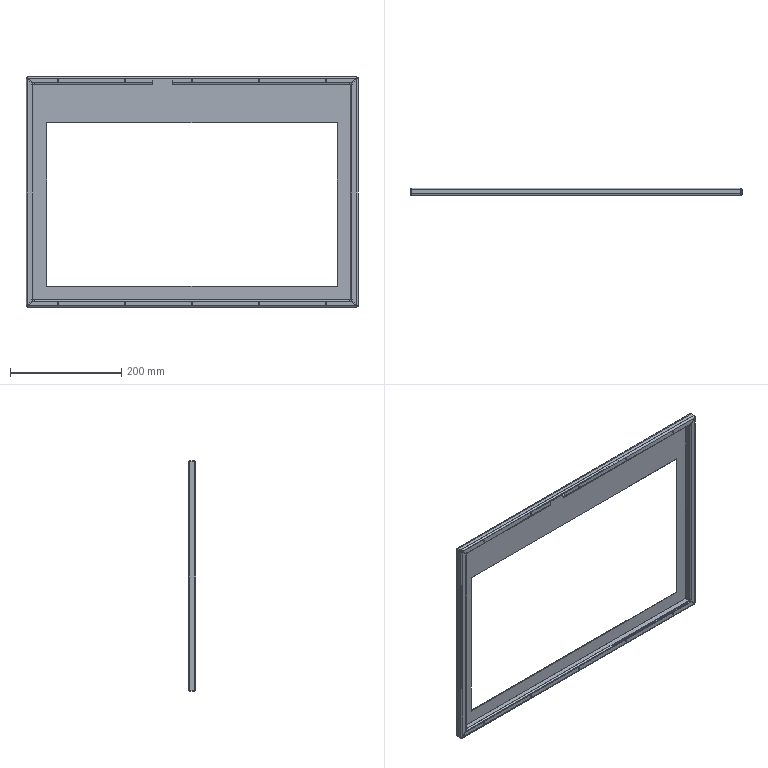Part | STEP file | 23.6 inch transparent screen frame 001 | 1 solid | 162 faces | box 596 x 13.5 x 414 mm | volume 232160 mm3 | plane 100 | cylinder 46 | spline 16 | commonest cylinder face diameters 2.5 x20 3 x13 6 x13